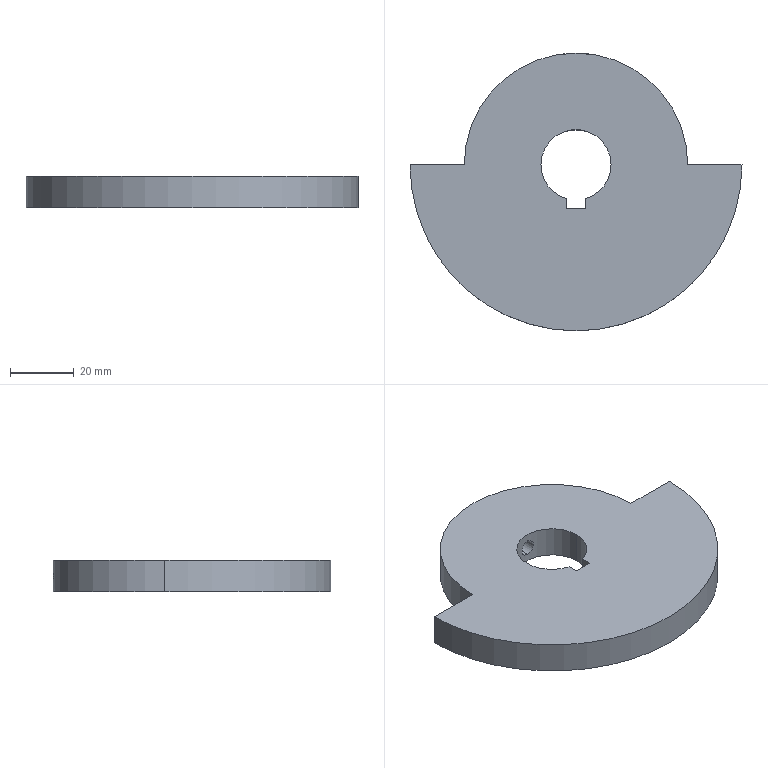Part | SolidWorks | features BaseBody 1 | 1 solid | 14 faces | box 104 x 87 x 10 mm | volume 57267 mm3 | cylinder 7 | plane 7 | commonest cylinder face diameters 22 x3 5 x2 70 x1 104 x1
STEP:
#1=CARTESIAN_POINT('',(11.,0.,5.));
#2=VERTEX_POINT('',#1);
#3=CARTESIAN_POINT('',(3.,-10.583,5.));
#4=VERTEX_POINT('',#3);
#5=CARTESIAN_POINT('',(0.,0.,5.));
#6=DIRECTION('',(0.,0.,-1.));
#7=DIRECTION('',(-1.,0.,0.));
#8=AXIS2_PLACEMENT_3D('',#5,#6,#7);
#9=CIRCLE('',#8,11.);
#10=EDGE_CURVE('',#2,#4,#9,.T.);
#11=ORIENTED_EDGE('',*,*,#10,.F.);
#12=CARTESIAN_POINT('',(11.,0.,-5.));
#13=VERTEX_POINT('',#12);
#14=CARTESIAN_POINT('',(11.,0.,5.));
#15=DIRECTION('',(0.,0.,-1.));
#16=VECTOR('',#15,1000.);
#17=LINE('',#14,#16);
#18=EDGE_CURVE('',#2,#13,#17,.T.);
#19=ORIENTED_EDGE('',*,*,#18,.T.);
#20=CARTESIAN_POINT('',(3.,-10.583,-5.));
#21=VERTEX_POINT('',#20);
#22=CARTESIAN_POINT('',(0.,0.,-5.));
#23=DIRECTION('',(0.,0.,1.));
#24=DIRECTION('',(-1.,0.,0.));
#25=AXIS2_PLACEMENT_3D('',#22,#23,#24);
#26=CIRCLE('',#25,11.);
#27=EDGE_CURVE('',#21,#13,#26,.T.);
#28=ORIENTED_EDGE('',*,*,#27,.F.);
#29=CARTESIAN_POINT('',(3.,-10.583,5.));
#30=DIRECTION('',(0.,0.,-1.));
#31=VECTOR('',#30,1000.);
#32=LINE('',#29,#31);
#33=EDGE_CURVE('',#4,#21,#32,.T.);
#34=ORIENTED_EDGE('',*,*,#33,.F.);
#35=EDGE_LOOP('',(#11,#19,#28,#34));
#36=FACE_OUTER_BOUND('',#35,.T.);
#37=CARTESIAN_POINT('',(0.,0.,5.));
#38=DIRECTION('',(0.,0.,-1.));
#39=DIRECTION('',(-1.,0.,0.));
#40=AXIS2_PLACEMENT_3D('',#37,#38,#39);
#41=CYLINDRICAL_SURFACE('',#40,11.);
#42=ADVANCED_FACE('',(#36),#41,.F.);
#43=ORIENTED_EDGE('',*,*,#18,.F.);
#44=CARTESIAN_POINT('',(-11.,0.,5.));
#45=VERTEX_POINT('',#44);
#46=CARTESIAN_POINT('',(0.,0.,5.));
#47=DIRECTION('',(0.,0.,-1.));
#48=DIRECTION('',(-1.,0.,0.));
#49=AXIS2_PLACEMENT_3D('',#46,#47,#48);
#50=CIRCLE('',#49,11.);
#51=EDGE_CURVE('',#45,#2,#50,.T.);
#52=ORIENTED_EDGE('',*,*,#51,.F.);
#53=CARTESIAN_POINT('',(-11.,0.,-5.));
#54=VERTEX_POINT('',#53);
#55=CARTESIAN_POINT('',(-11.,0.,5.));
#56=DIRECTION('',(0.,0.,-1.));
#57=VECTOR('',#56,1000.);
#58=LINE('',#55,#57);
#59=EDGE_CURVE('',#45,#54,#58,.T.);
#60=ORIENTED_EDGE('',*,*,#59,.T.);
#61=CARTESIAN_POINT('',(0.,0.,-5.));
#62=DIRECTION('',(0.,0.,1.));
#63=DIRECTION('',(-1.,0.,0.));
#64=AXIS2_PLACEMENT_3D('',#61,#62,#63);
#65=CIRCLE('',#64,11.);
#66=EDGE_CURVE('',#13,#54,#65,.T.);
#67=ORIENTED_EDGE('',*,*,#66,.F.);
#68=EDGE_LOOP('',(#43,#52,#60,#67));
#69=FACE_OUTER_BOUND('',#68,.T.);
#70=CARTESIAN_POINT('',(0.,11.,-2.5));
#71=VERTEX_POINT('',#70);
#72=CARTESIAN_POINT('',(0.,11.,2.5));
#73=VERTEX_POINT('',#72);
#74=CARTESIAN_POINT('',(0.,11.,-2.5));
#75=CARTESIAN_POINT('',(0.1657,11.,-2.5));
#76=CARTESIAN_POINT('',(0.3286,10.996,-2.484));
#77=CARTESIAN_POINT('',(0.6488,10.982,-2.42));
#78=CARTESIAN_POINT('',(0.8078,10.971,-2.372));
#79=CARTESIAN_POINT('',(1.11,10.945,-2.246));
#80=CARTESIAN_POINT('',(1.254,10.929,-2.169));
#81=CARTESIAN_POINT('',(1.525,10.895,-1.988));
#82=CARTESIAN_POINT('',(1.653,10.876,-1.883));
#83=CARTESIAN_POINT('',(1.998,10.82,-1.538));
#84=CARTESIAN_POINT('',(2.184,10.782,-1.26));
#85=CARTESIAN_POINT('',(2.371,10.742,-0.8093));
#86=CARTESIAN_POINT('',(2.419,10.731,-0.6512));
#87=CARTESIAN_POINT('',(2.484,10.716,-0.3283));
#88=CARTESIAN_POINT('',(2.5,10.712,-0.1658));
#89=CARTESIAN_POINT('',(2.5,10.712,0.1615));
#90=CARTESIAN_POINT('',(2.484,10.716,0.3277));
#91=CARTESIAN_POINT('',(2.42,10.731,0.6487));
#92=CARTESIAN_POINT('',(2.373,10.741,0.8048));
#93=CARTESIAN_POINT('',(2.184,10.782,1.26));
#94=CARTESIAN_POINT('',(2.,10.819,1.535));
#95=CARTESIAN_POINT('',(1.653,10.876,1.883));
#96=CARTESIAN_POINT('',(1.527,10.894,1.986));
#97=CARTESIAN_POINT('',(1.257,10.929,2.167));
#98=CARTESIAN_POINT('',(1.111,10.945,2.246));
#99=CARTESIAN_POINT('',(0.8089,10.971,2.371));
#100=CARTESIAN_POINT('',(0.6531,10.982,2.419));
#101=CARTESIAN_POINT('',(0.3316,10.996,2.483));
#102=CARTESIAN_POINT('',(0.1657,11.,2.5));
#103=CARTESIAN_POINT('',(0.,11.,2.5));
#104=B_SPLINE_CURVE_WITH_KNOTS('',3,(#74,#75,#76,#77,#78,#79,#80,#81,#82,#83,#84,#85,#86,#87,#88,#89,#90,#91,#92,#93,#94,#95,#96,#97,#98,#99,#100,#101,#102,#103),.UNSPECIFIED.,.F.,.F.,(4,2,2,2,2,2,2,2,2,2,2,2,2,2,4),(0.,0.00049,0.0009799,0.00147,0.00196,0.00294,0.00343,0.00392,0.00441,0.0049,0.00588,0.00637,0.00686,0.00735,0.00784),.UNSPECIFIED.);
#105=EDGE_CURVE('',#71,#73,#104,.T.);
#106=ORIENTED_EDGE('',*,*,#105,.F.);
#107=CARTESIAN_POINT('',(0.,11.,2.5));
#108=CARTESIAN_POINT('',(-0.1657,11.,2.5));
#109=CARTESIAN_POINT('',(-0.3286,10.996,2.484));
#110=CARTESIAN_POINT('',(-0.6488,10.982,2.42));
#111=CARTESIAN_POINT('',(-0.8078,10.971,2.372));
#112=CARTESIAN_POINT('',(-1.11,10.945,2.246));
#113=CARTESIAN_POINT('',(-1.254,10.929,2.169));
#114=CARTESIAN_POINT('',(-1.525,10.895,1.988));
#115=CARTESIAN_POINT('',(-1.653,10.876,1.883));
#116=CARTESIAN_POINT('',(-1.998,10.82,1.538));
#117=CARTESIAN_POINT('',(-2.184,10.782,1.26));
#118=CARTESIAN_POINT('',(-2.371,10.742,0.8093));
#119=CARTESIAN_POINT('',(-2.419,10.731,0.6512));
#120=CARTESIAN_POINT('',(-2.484,10.716,0.3283));
#121=CARTESIAN_POINT('',(-2.5,10.712,0.1658));
#122=CARTESIAN_POINT('',(-2.5,10.712,-0.1615));
#123=CARTESIAN_POINT('',(-2.484,10.716,-0.3277));
#124=CARTESIAN_POINT('',(-2.42,10.731,-0.6487));
#125=CARTESIAN_POINT('',(-2.373,10.741,-0.8048));
#126=CARTESIAN_POINT('',(-2.184,10.782,-1.26));
#127=CARTESIAN_POINT('',(-2.,10.819,-1.535));
#128=CARTESIAN_POINT('',(-1.653,10.876,-1.883));
#129=CARTESIAN_POINT('',(-1.527,10.894,-1.986));
#130=CARTESIAN_POINT('',(-1.257,10.929,-2.167));
#131=CARTESIAN_POINT('',(-1.111,10.945,-2.246));
#132=CARTESIAN_POINT('',(-0.8089,10.971,-2.371));
#133=CARTESIAN_POINT('',(-0.6531,10.982,-2.419));
#134=CARTESIAN_POINT('',(-0.3316,10.996,-2.483));
#135=CARTESIAN_POINT('',(-0.1657,11.,-2.5));
#136=CARTESIAN_POINT('',(0.,11.,-2.5));
#137=B_SPLINE_CURVE_WITH_KNOTS('',3,(#107,#108,#109,#110,#111,#112,#113,#114,#115,#116,#117,#118,#119,#120,#121,#122,#123,#124,#125,#126,#127,#128,#129,#130,#131,#132,#133,#134,#135,#136),.UNSPECIFIED.,.F.,.F.,(4,2,2,2,2,2,2,2,2,2,2,2,2,2,4),(0.00784,0.00833,0.008819,0.009309,0.009799,0.01078,0.01127,0.01176,0.01225,0.01274,0.01372,0.01421,0.0147,0.01519,0.01568),.UNSPECIFIED.);
#138=EDGE_CURVE('',#73,#71,#137,.T.);
#139=ORIENTED_EDGE('',*,*,#138,.F.);
#140=EDGE_LOOP('',(#106,#139));
#141=FACE_BOUND('',#140,.T.);
#142=CARTESIAN_POINT('',(0.,0.,5.));
#143=DIRECTION('',(0.,0.,-1.));
#144=DIRECTION('',(-1.,0.,0.));
#145=AXIS2_PLACEMENT_3D('',#142,#143,#144);
#146=CYLINDRICAL_SURFACE('',#145,11.);
#147=ADVANCED_FACE('',(#69,#141),#146,.F.);
#148=CARTESIAN_POINT('',(0.,35.,2.5));
#149=VERTEX_POINT('',#148);
#150=CARTESIAN_POINT('',(0.,35.,-2.5));
#151=VERTEX_POINT('',#150);
#152=CARTESIAN_POINT('',(0.,35.,2.5));
#153=CARTESIAN_POINT('',(-0.1652,35.,2.5));
#154=CARTESIAN_POINT('',(-0.3276,34.999,2.484));
#155=CARTESIAN_POINT('',(-0.6472,34.994,2.42));
#156=CARTESIAN_POINT('',(-0.806,34.991,2.372));
#157=CARTESIAN_POINT('',(-1.109,34.983,2.247));
#158=CARTESIAN_POINT('',(-1.252,34.978,2.17));
#159=CARTESIAN_POINT('',(-1.524,34.967,1.989));
#160=CARTESIAN_POINT('',(-1.653,34.961,1.883));
#161=CARTESIAN_POINT('',(-1.883,34.949,1.652));
#162=CARTESIAN_POINT('',(-1.987,34.944,1.527));
#163=CARTESIAN_POINT('',(-2.169,34.933,1.253));
#164=CARTESIAN_POINT('',(-2.247,34.928,1.108));
#165=CARTESIAN_POINT('',(-2.372,34.92,0.8073));
#166=CARTESIAN_POINT('',(-2.42,34.916,0.6497));
#167=CARTESIAN_POINT('',(-2.484,34.912,0.327));
#168=CARTESIAN_POINT('',(-2.5,34.911,0.1648));
#169=CARTESIAN_POINT('',(-2.5,34.911,-0.1613));
#170=CARTESIAN_POINT('',(-2.484,34.912,-0.327));
#171=CARTESIAN_POINT('',(-2.42,34.916,-0.6477));
#172=CARTESIAN_POINT('',(-2.373,34.92,-0.8035));
#173=CARTESIAN_POINT('',(-2.248,34.928,-1.106));
#174=CARTESIAN_POINT('',(-2.17,34.933,-1.253));
#175=CARTESIAN_POINT('',(-1.989,34.944,-1.523));
#176=CARTESIAN_POINT('',(-1.886,34.949,-1.65));
#177=CARTESIAN_POINT('',(-1.652,34.961,-1.883));
#178=CARTESIAN_POINT('',(-1.526,34.967,-1.987));
#179=CARTESIAN_POINT('',(-1.256,34.978,-2.168));
#180=CARTESIAN_POINT('',(-1.109,34.983,-2.246));
#181=CARTESIAN_POINT('',(-0.8067,34.991,-2.372));
#182=CARTESIAN_POINT('',(-0.6509,34.994,-2.419));
#183=CARTESIAN_POINT('',(-0.3305,34.999,-2.483));
#184=CARTESIAN_POINT('',(-0.1652,35.,-2.5));
#185=CARTESIAN_POINT('',(0.,35.,-2.5));
#186=B_SPLINE_CURVE_WITH_KNOTS('',3,(#152,#153,#154,#155,#156,#157,#158,#159,#160,#161,#162,#163,#164,#165,#166,#167,#168,#169,#170,#171,#172,#173,#174,#175,#176,#177,#178,#179,#180,#181,#182,#183,#184,#185),.UNSPECIFIED.,.F.,.F.,(4,2,2,2,2,2,2,2,2,2,2,2,2,2,2,2,4),(0.,0.0004886,0.0009771,0.001466,0.001954,0.002443,0.002931,0.00342,0.003908,0.004397,0.004886,0.005374,0.005863,0.006351,0.00684,0.007328,0.007817),.UNSPECIFIED.);
#187=EDGE_CURVE('',#149,#151,#186,.T.);
#188=ORIENTED_EDGE('',*,*,#187,.F.);
#189=CARTESIAN_POINT('',(0.,0.,2.5));
#190=DIRECTION('',(0.,-1.,0.));
#191=VECTOR('',#190,1000.);
#192=LINE('',#189,#191);
#193=EDGE_CURVE('',#149,#73,#192,.T.);
#194=ORIENTED_EDGE('',*,*,#193,.T.);
#195=ORIENTED_EDGE('',*,*,#138,.T.);
#196=CARTESIAN_POINT('',(0.,0.,-2.5));
#197=DIRECTION('',(0.,-1.,0.));
#198=VECTOR('',#197,1000.);
#199=LINE('',#196,#198);
#200=EDGE_CURVE('',#151,#71,#199,.T.);
#201=ORIENTED_EDGE('',*,*,#200,.F.);
#202=EDGE_LOOP('',(#188,#194,#195,#201));
#203=FACE_OUTER_BOUND('',#202,.T.);
#204=CARTESIAN_POINT('',(0.,0.,0.));
#205=DIRECTION('',(0.,-1.,0.));
#206=DIRECTION('',(0.,0.,-1.));
#207=AXIS2_PLACEMENT_3D('',#204,#205,#206);
#208=CYLINDRICAL_SURFACE('',#207,2.5);
#209=ADVANCED_FACE('',(#203),#208,.F.);
#210=CARTESIAN_POINT('',(35.,0.,5.));
#211=VERTEX_POINT('',#210);
#212=CARTESIAN_POINT('',(-35.,0.,5.));
#213=VERTEX_POINT('',#212);
#214=CARTESIAN_POINT('',(0.,0.,5.));
#215=DIRECTION('',(0.,0.,1.));
#216=DIRECTION('',(-1.,0.,0.));
#217=AXIS2_PLACEMENT_3D('',#214,#215,#216);
#218=CIRCLE('',#217,35.);
#219=EDGE_CURVE('',#211,#213,#218,.T.);
#220=ORIENTED_EDGE('',*,*,#219,.T.);
#221=CARTESIAN_POINT('',(-52.,0.,5.));
#222=VERTEX_POINT('',#221);
#223=CARTESIAN_POINT('',(0.,0.,5.));
#224=DIRECTION('',(-1.,0.,0.));
#225=VECTOR('',#224,1000.);
#226=LINE('',#223,#225);
#227=EDGE_CURVE('',#213,#222,#226,.T.);
#228=ORIENTED_EDGE('',*,*,#227,.T.);
#229=CARTESIAN_POINT('',(52.,0.,5.));
#230=VERTEX_POINT('',#229);
#231=CARTESIAN_POINT('',(0.,0.,5.));
#232=DIRECTION('',(0.,0.,1.));
#233=DIRECTION('',(-1.,0.,0.));
#234=AXIS2_PLACEMENT_3D('',#231,#232,#233);
#235=CIRCLE('',#234,52.);
#236=EDGE_CURVE('',#222,#230,#235,.T.);
#237=ORIENTED_EDGE('',*,*,#236,.T.);
#238=CARTESIAN_POINT('',(0.,0.,5.));
#239=DIRECTION('',(-1.,0.,0.));
#240=VECTOR('',#239,1000.);
#241=LINE('',#238,#240);
#242=EDGE_CURVE('',#230,#211,#241,.T.);
#243=ORIENTED_EDGE('',*,*,#242,.T.);
#244=EDGE_LOOP('',(#220,#228,#237,#243));
#245=FACE_OUTER_BOUND('',#244,.T.);
#246=CARTESIAN_POINT('',(-3.,-10.583,5.));
#247=VERTEX_POINT('',#246);
#248=CARTESIAN_POINT('',(0.,0.,5.));
#249=DIRECTION('',(0.,0.,-1.));
#250=DIRECTION('',(-1.,0.,0.));
#251=AXIS2_PLACEMENT_3D('',#248,#249,#250);
#252=CIRCLE('',#251,11.);
#253=EDGE_CURVE('',#247,#45,#252,.T.);
#254=ORIENTED_EDGE('',*,*,#253,.T.);
#255=ORIENTED_EDGE('',*,*,#51,.T.);
#256=ORIENTED_EDGE('',*,*,#10,.T.);
#257=CARTESIAN_POINT('',(3.,-13.8,5.));
#258=VERTEX_POINT('',#257);
#259=CARTESIAN_POINT('',(3.,0.,5.));
#260=DIRECTION('',(0.,-1.,0.));
#261=VECTOR('',#260,1000.);
#262=LINE('',#259,#261);
#263=EDGE_CURVE('',#4,#258,#262,.T.);
#264=ORIENTED_EDGE('',*,*,#263,.T.);
#265=CARTESIAN_POINT('',(-3.,-13.8,5.));
#266=VERTEX_POINT('',#265);
#267=CARTESIAN_POINT('',(0.,-13.8,5.));
#268=DIRECTION('',(-1.,0.,0.));
#269=VECTOR('',#268,1000.);
#270=LINE('',#267,#269);
#271=EDGE_CURVE('',#258,#266,#270,.T.);
#272=ORIENTED_EDGE('',*,*,#271,.T.);
#273=CARTESIAN_POINT('',(-3.,0.,5.));
#274=DIRECTION('',(0.,1.,0.));
#275=VECTOR('',#274,1000.);
#276=LINE('',#273,#275);
#277=EDGE_CURVE('',#266,#247,#276,.T.);
#278=ORIENTED_EDGE('',*,*,#277,.T.);
#279=EDGE_LOOP('',(#254,#255,#256,#264,#272,#278));
#280=FACE_BOUND('',#279,.T.);
#281=CARTESIAN_POINT('',(0.,0.,5.));
#282=DIRECTION('',(0.,0.,1.));
#283=DIRECTION('',(1.,0.,0.));
#284=AXIS2_PLACEMENT_3D('',#281,#282,#283);
#285=PLANE('',#284);
#286=ADVANCED_FACE('',(#245,#280),#285,.T.);
#287=CARTESIAN_POINT('',(-52.,0.,-5.));
#288=VERTEX_POINT('',#287);
#289=CARTESIAN_POINT('',(-52.,0.,5.));
#290=DIRECTION('',(0.,0.,-1.));
#291=VECTOR('',#290,1000.);
#292=LINE('',#289,#291);
#293=EDGE_CURVE('',#222,#288,#292,.T.);
#294=ORIENTED_EDGE('',*,*,#293,.F.);
#295=ORIENTED_EDGE('',*,*,#227,.F.);
#296=CARTESIAN_POINT('',(-35.,0.,-5.));
#297=VERTEX_POINT('',#296);
#298=CARTESIAN_POINT('',(-35.,0.,5.));
#299=DIRECTION('',(0.,0.,1.));
#300=VECTOR('',#299,1000.);
#301=LINE('',#298,#300);
#302=EDGE_CURVE('',#297,#213,#301,.T.);
#303=ORIENTED_EDGE('',*,*,#302,.F.);
#304=CARTESIAN_POINT('',(-52.,0.,-5.));
#305=DIRECTION('',(1.,0.,0.));
#306=VECTOR('',#305,1000.);
#307=LINE('',#304,#306);
#308=EDGE_CURVE('',#288,#297,#307,.T.);
#309=ORIENTED_EDGE('',*,*,#308,.F.);
#310=EDGE_LOOP('',(#294,#295,#303,#309));
#311=FACE_OUTER_BOUND('',#310,.T.);
#312=CARTESIAN_POINT('',(-52.,0.,5.));
#313=DIRECTION('',(0.,-1.,0.));
#314=DIRECTION('',(0.,0.,-1.));
#315=AXIS2_PLACEMENT_3D('',#312,#313,#314);
#316=PLANE('',#315);
#317=ADVANCED_FACE('',(#311),#316,.F.);
#318=ORIENTED_EDGE('',*,*,#219,.F.);
#319=CARTESIAN_POINT('',(35.,0.,-5.));
#320=VERTEX_POINT('',#319);
#321=CARTESIAN_POINT('',(35.,0.,5.));
#322=DIRECTION('',(0.,0.,-1.));
#323=VECTOR('',#322,1000.);
#324=LINE('',#321,#323);
#325=EDGE_CURVE('',#211,#320,#324,.T.);
#326=ORIENTED_EDGE('',*,*,#325,.T.);
#327=CARTESIAN_POINT('',(0.,0.,-5.));
#328=DIRECTION('',(0.,0.,1.));
#329=DIRECTION('',(-1.,0.,0.));
#330=AXIS2_PLACEMENT_3D('',#327,#328,#329);
#331=CIRCLE('',#330,35.);
#332=EDGE_CURVE('',#320,#297,#331,.T.);
#333=ORIENTED_EDGE('',*,*,#332,.T.);
#334=ORIENTED_EDGE('',*,*,#302,.T.);
#335=EDGE_LOOP('',(#318,#326,#333,#334));
#336=FACE_OUTER_BOUND('',#335,.T.);
#337=CARTESIAN_POINT('',(0.,35.,-2.5));
#338=CARTESIAN_POINT('',(0.1652,35.,-2.5));
#339=CARTESIAN_POINT('',(0.3276,34.999,-2.484));
#340=CARTESIAN_POINT('',(0.6472,34.994,-2.42));
#341=CARTESIAN_POINT('',(0.806,34.991,-2.372));
#342=CARTESIAN_POINT('',(1.109,34.983,-2.247));
#343=CARTESIAN_POINT('',(1.252,34.978,-2.17));
#344=CARTESIAN_POINT('',(1.524,34.967,-1.989));
#345=CARTESIAN_POINT('',(1.653,34.961,-1.883));
#346=CARTESIAN_POINT('',(1.883,34.949,-1.652));
#347=CARTESIAN_POINT('',(1.987,34.944,-1.527));
#348=CARTESIAN_POINT('',(2.169,34.933,-1.253));
#349=CARTESIAN_POINT('',(2.247,34.928,-1.108));
#350=CARTESIAN_POINT('',(2.372,34.92,-0.8073));
#351=CARTESIAN_POINT('',(2.42,34.916,-0.6497));
#352=CARTESIAN_POINT('',(2.484,34.912,-0.327));
#353=CARTESIAN_POINT('',(2.5,34.911,-0.1648));
#354=CARTESIAN_POINT('',(2.5,34.911,0.1613));
#355=CARTESIAN_POINT('',(2.484,34.912,0.327));
#356=CARTESIAN_POINT('',(2.42,34.916,0.6477));
#357=CARTESIAN_POINT('',(2.373,34.92,0.8035));
#358=CARTESIAN_POINT('',(2.248,34.928,1.106));
#359=CARTESIAN_POINT('',(2.17,34.933,1.253));
#360=CARTESIAN_POINT('',(1.989,34.944,1.523));
#361=CARTESIAN_POINT('',(1.886,34.949,1.65));
#362=CARTESIAN_POINT('',(1.652,34.961,1.883));
#363=CARTESIAN_POINT('',(1.526,34.967,1.987));
#364=CARTESIAN_POINT('',(1.256,34.978,2.168));
#365=CARTESIAN_POINT('',(1.109,34.983,2.246));
#366=CARTESIAN_POINT('',(0.8067,34.991,2.372));
#367=CARTESIAN_POINT('',(0.6509,34.994,2.419));
#368=CARTESIAN_POINT('',(0.3305,34.999,2.483));
#369=CARTESIAN_POINT('',(0.1652,35.,2.5));
#370=CARTESIAN_POINT('',(0.,35.,2.5));
#371=B_SPLINE_CURVE_WITH_KNOTS('',3,(#337,#338,#339,#340,#341,#342,#343,#344,#345,#346,#347,#348,#349,#350,#351,#352,#353,#354,#355,#356,#357,#358,#359,#360,#361,#362,#363,#364,#365,#366,#367,#368,#369,#370),.UNSPECIFIED.,.F.,.F.,(4,2,2,2,2,2,2,2,2,2,2,2,2,2,2,2,4),(0.007817,0.008306,0.008794,0.009283,0.009771,0.01026,0.01075,0.01124,0.01173,0.01221,0.0127,0.01319,0.01368,0.01417,0.01466,0.01515,0.01563),.UNSPECIFIED.);
#372=EDGE_CURVE('',#151,#149,#371,.T.);
#373=ORIENTED_EDGE('',*,*,#372,.T.);
#374=ORIENTED_EDGE('',*,*,#187,.T.);
#375=EDGE_LOOP('',(#373,#374));
#376=FACE_BOUND('',#375,.T.);
#377=CARTESIAN_POINT('',(0.,0.,5.));
#378=DIRECTION('',(0.,0.,-1.));
#379=DIRECTION('',(-1.,0.,0.));
#380=AXIS2_PLACEMENT_3D('',#377,#378,#379);
#381=CYLINDRICAL_SURFACE('',#380,35.);
#382=ADVANCED_FACE('',(#336,#376),#381,.T.);
#383=ORIENTED_EDGE('',*,*,#325,.F.);
#384=ORIENTED_EDGE('',*,*,#242,.F.);
#385=CARTESIAN_POINT('',(52.,0.,-5.));
#386=VERTEX_POINT('',#385);
#387=CARTESIAN_POINT('',(52.,0.,5.));
#388=DIRECTION('',(0.,0.,1.));
#389=VECTOR('',#388,1000.);
#390=LINE('',#387,#389);
#391=EDGE_CURVE('',#386,#230,#390,.T.);
#392=ORIENTED_EDGE('',*,*,#391,.F.);
#393=CARTESIAN_POINT('',(35.,0.,-5.));
#394=DIRECTION('',(1.,0.,0.));
#395=VECTOR('',#394,1000.);
#396=LINE('',#393,#395);
#397=EDGE_CURVE('',#320,#386,#396,.T.);
#398=ORIENTED_EDGE('',*,*,#397,.F.);
#399=EDGE_LOOP('',(#383,#384,#392,#398));
#400=FACE_OUTER_BOUND('',#399,.T.);
#401=CARTESIAN_POINT('',(35.,0.,5.));
#402=DIRECTION('',(0.,-1.,0.));
#403=DIRECTION('',(0.,0.,-1.));
#404=AXIS2_PLACEMENT_3D('',#401,#402,#403);
#405=PLANE('',#404);
#406=ADVANCED_FACE('',(#400),#405,.F.);
#407=ORIENTED_EDGE('',*,*,#236,.F.);
#408=ORIENTED_EDGE('',*,*,#293,.T.);
#409=CARTESIAN_POINT('',(0.,0.,-5.));
#410=DIRECTION('',(0.,0.,1.));
#411=DIRECTION('',(-1.,0.,0.));
#412=AXIS2_PLACEMENT_3D('',#409,#410,#411);
#413=CIRCLE('',#412,52.);
#414=EDGE_CURVE('',#288,#386,#413,.T.);
#415=ORIENTED_EDGE('',*,*,#414,.T.);
#416=ORIENTED_EDGE('',*,*,#391,.T.);
#417=EDGE_LOOP('',(#407,#408,#415,#416));
#418=FACE_OUTER_BOUND('',#417,.T.);
#419=CARTESIAN_POINT('',(0.,0.,5.));
#420=DIRECTION('',(0.,0.,-1.));
#421=DIRECTION('',(-1.,0.,0.));
#422=AXIS2_PLACEMENT_3D('',#419,#420,#421);
#423=CYLINDRICAL_SURFACE('',#422,52.);
#424=ADVANCED_FACE('',(#418),#423,.T.);
#425=ORIENTED_EDGE('',*,*,#59,.F.);
#426=ORIENTED_EDGE('',*,*,#253,.F.);
#427=CARTESIAN_POINT('',(-3.,-10.583,-5.));
#428=VERTEX_POINT('',#427);
#429=CARTESIAN_POINT('',(-3.,-10.583,5.));
#430=DIRECTION('',(0.,0.,1.));
#431=VECTOR('',#430,1000.);
#432=LINE('',#429,#431);
#433=EDGE_CURVE('',#428,#247,#432,.T.);
#434=ORIENTED_EDGE('',*,*,#433,.F.);
#435=CARTESIAN_POINT('',(0.,0.,-5.));
#436=DIRECTION('',(0.,0.,1.));
#437=DIRECTION('',(-1.,0.,0.));
#438=AXIS2_PLACEMENT_3D('',#435,#436,#437);
#439=CIRCLE('',#438,11.);
#440=EDGE_CURVE('',#54,#428,#439,.T.);
#441=ORIENTED_EDGE('',*,*,#440,.F.);
#442=EDGE_LOOP('',(#425,#426,#434,#441));
#443=FACE_OUTER_BOUND('',#442,.T.);
#444=CARTESIAN_POINT('',(0.,0.,5.));
#445=DIRECTION('',(0.,0.,-1.));
#446=DIRECTION('',(-1.,0.,0.));
#447=AXIS2_PLACEMENT_3D('',#444,#445,#446);
#448=CYLINDRICAL_SURFACE('',#447,11.);
#449=ADVANCED_FACE('',(#443),#448,.F.);
#450=ORIENTED_EDGE('',*,*,#277,.F.);
#451=CARTESIAN_POINT('',(-3.,-13.8,-5.));
#452=VERTEX_POINT('',#451);
#453=CARTESIAN_POINT('',(-3.,-13.8,-5.));
#454=DIRECTION('',(0.,0.,1.));
#455=VECTOR('',#454,1000.);
#456=LINE('',#453,#455);
#457=EDGE_CURVE('',#452,#266,#456,.T.);
#458=ORIENTED_EDGE('',*,*,#457,.F.);
#459=CARTESIAN_POINT('',(-3.,-13.8,-5.));
#460=DIRECTION('',(0.,-1.,0.));
#461=VECTOR('',#460,1000.);
#462=LINE('',#459,#461);
#463=EDGE_CURVE('',#428,#452,#462,.T.);
#464=ORIENTED_EDGE('',*,*,#463,.F.);
#465=ORIENTED_EDGE('',*,*,#433,.T.);
#466=EDGE_LOOP('',(#450,#458,#464,#465));
#467=FACE_OUTER_BOUND('',#466,.T.);
#468=CARTESIAN_POINT('',(-3.,-13.8,-5.));
#469=DIRECTION('',(-1.,0.,0.));
#470=DIRECTION('',(0.,0.,1.));
#471=AXIS2_PLACEMENT_3D('',#468,#469,#470);
#472=PLANE('',#471);
#473=ADVANCED_FACE('',(#467),#472,.F.);
#474=CARTESIAN_POINT('',(3.,-13.8,-5.));
#475=VERTEX_POINT('',#474);
#476=CARTESIAN_POINT('',(3.,-13.8,-5.));
#477=DIRECTION('',(0.,0.,1.));
#478=VECTOR('',#477,1000.);
#479=LINE('',#476,#478);
#480=EDGE_CURVE('',#475,#258,#479,.T.);
#481=ORIENTED_EDGE('',*,*,#480,.F.);
#482=CARTESIAN_POINT('',(-3.,-13.8,-5.));
#483=DIRECTION('',(1.,0.,0.));
#484=VECTOR('',#483,1000.);
#485=LINE('',#482,#484);
#486=EDGE_CURVE('',#452,#475,#485,.T.);
#487=ORIENTED_EDGE('',*,*,#486,.F.);
#488=ORIENTED_EDGE('',*,*,#457,.T.);
#489=ORIENTED_EDGE('',*,*,#271,.F.);
#490=EDGE_LOOP('',(#481,#487,#488,#489));
#491=FACE_OUTER_BOUND('',#490,.T.);
#492=CARTESIAN_POINT('',(-3.,-13.8,-5.));
#493=DIRECTION('',(0.,-1.,0.));
#494=DIRECTION('',(0.,0.,-1.));
#495=AXIS2_PLACEMENT_3D('',#492,#493,#494);
#496=PLANE('',#495);
#497=ADVANCED_FACE('',(#491),#496,.F.);
#498=CARTESIAN_POINT('',(3.,-13.8,-5.));
#499=DIRECTION('',(0.,1.,0.));
#500=VECTOR('',#499,1000.);
#501=LINE('',#498,#500);
#502=EDGE_CURVE('',#475,#21,#501,.T.);
#503=ORIENTED_EDGE('',*,*,#502,.F.);
#504=ORIENTED_EDGE('',*,*,#480,.T.);
#505=ORIENTED_EDGE('',*,*,#263,.F.);
#506=ORIENTED_EDGE('',*,*,#33,.T.);
#507=EDGE_LOOP('',(#503,#504,#505,#506));
#508=FACE_OUTER_BOUND('',#507,.T.);
#509=CARTESIAN_POINT('',(3.,-13.8,-5.));
#510=DIRECTION('',(1.,0.,0.));
#511=DIRECTION('',(0.,0.,-1.));
#512=AXIS2_PLACEMENT_3D('',#509,#510,#511);
#513=PLANE('',#512);
#514=ADVANCED_FACE('',(#508),#513,.F.);
#515=ORIENTED_EDGE('',*,*,#502,.T.);
#516=ORIENTED_EDGE('',*,*,#27,.T.);
#517=ORIENTED_EDGE('',*,*,#66,.T.);
#518=ORIENTED_EDGE('',*,*,#440,.T.);
#519=ORIENTED_EDGE('',*,*,#463,.T.);
#520=ORIENTED_EDGE('',*,*,#486,.T.);
#521=EDGE_LOOP('',(#515,#516,#517,#518,#519,#520));
#522=FACE_BOUND('',#521,.T.);
#523=ORIENTED_EDGE('',*,*,#308,.T.);
#524=ORIENTED_EDGE('',*,*,#332,.F.);
#525=ORIENTED_EDGE('',*,*,#397,.T.);
#526=ORIENTED_EDGE('',*,*,#414,.F.);
#527=EDGE_LOOP('',(#523,#524,#525,#526));
#528=FACE_OUTER_BOUND('',#527,.T.);
#529=CARTESIAN_POINT('',(0.,0.,-5.));
#530=DIRECTION('',(0.,0.,1.));
#531=DIRECTION('',(1.,0.,0.));
#532=AXIS2_PLACEMENT_3D('',#529,#530,#531);
#533=PLANE('',#532);
#534=ADVANCED_FACE('',(#522,#528),#533,.F.);
#535=ORIENTED_EDGE('',*,*,#193,.F.);
#536=ORIENTED_EDGE('',*,*,#372,.F.);
#537=ORIENTED_EDGE('',*,*,#200,.T.);
#538=ORIENTED_EDGE('',*,*,#105,.T.);
#539=EDGE_LOOP('',(#535,#536,#537,#538));
#540=FACE_OUTER_BOUND('',#539,.T.);
#541=CARTESIAN_POINT('',(0.,0.,0.));
#542=DIRECTION('',(0.,-1.,0.));
#543=DIRECTION('',(0.,0.,-1.));
#544=AXIS2_PLACEMENT_3D('',#541,#542,#543);
#545=CYLINDRICAL_SURFACE('',#544,2.5);
#546=ADVANCED_FACE('',(#540),#545,.F.);
#547=CLOSED_SHELL('',(#42,#147,#209,#286,#317,#382,#406,#424,#449,#473,#497,#514,#534,#546));
#548=MANIFOLD_SOLID_BREP('',#547);
#549=CARTESIAN_POINT('',(0.,0.,0.));
#550=DIRECTION('',(0.,0.,1.));
#551=DIRECTION('',(1.,0.,0.));
#552=AXIS2_PLACEMENT_3D('',#549,#550,#551);
#553=(LENGTH_UNIT()NAMED_UNIT(*)SI_UNIT(.MILLI.,.METRE.));
#554=UNCERTAINTY_MEASURE_WITH_UNIT(LENGTH_MEASURE(0.00001),#553,'','');
#555=(NAMED_UNIT(*)PLANE_ANGLE_UNIT()SI_UNIT($,.RADIAN.));
#556=(NAMED_UNIT(*)SI_UNIT($,.STERADIAN.)SOLID_ANGLE_UNIT());
#557=(GEOMETRIC_REPRESENTATION_CONTEXT(3)GLOBAL_UNCERTAINTY_ASSIGNED_CONTEXT((#554))GLOBAL_UNIT_ASSIGNED_CONTEXT((#553,#555,#556))REPRESENTATION_CONTEXT('',''));
#558=ADVANCED_BREP_SHAPE_REPRESENTATION('',(#548,#552),#557);